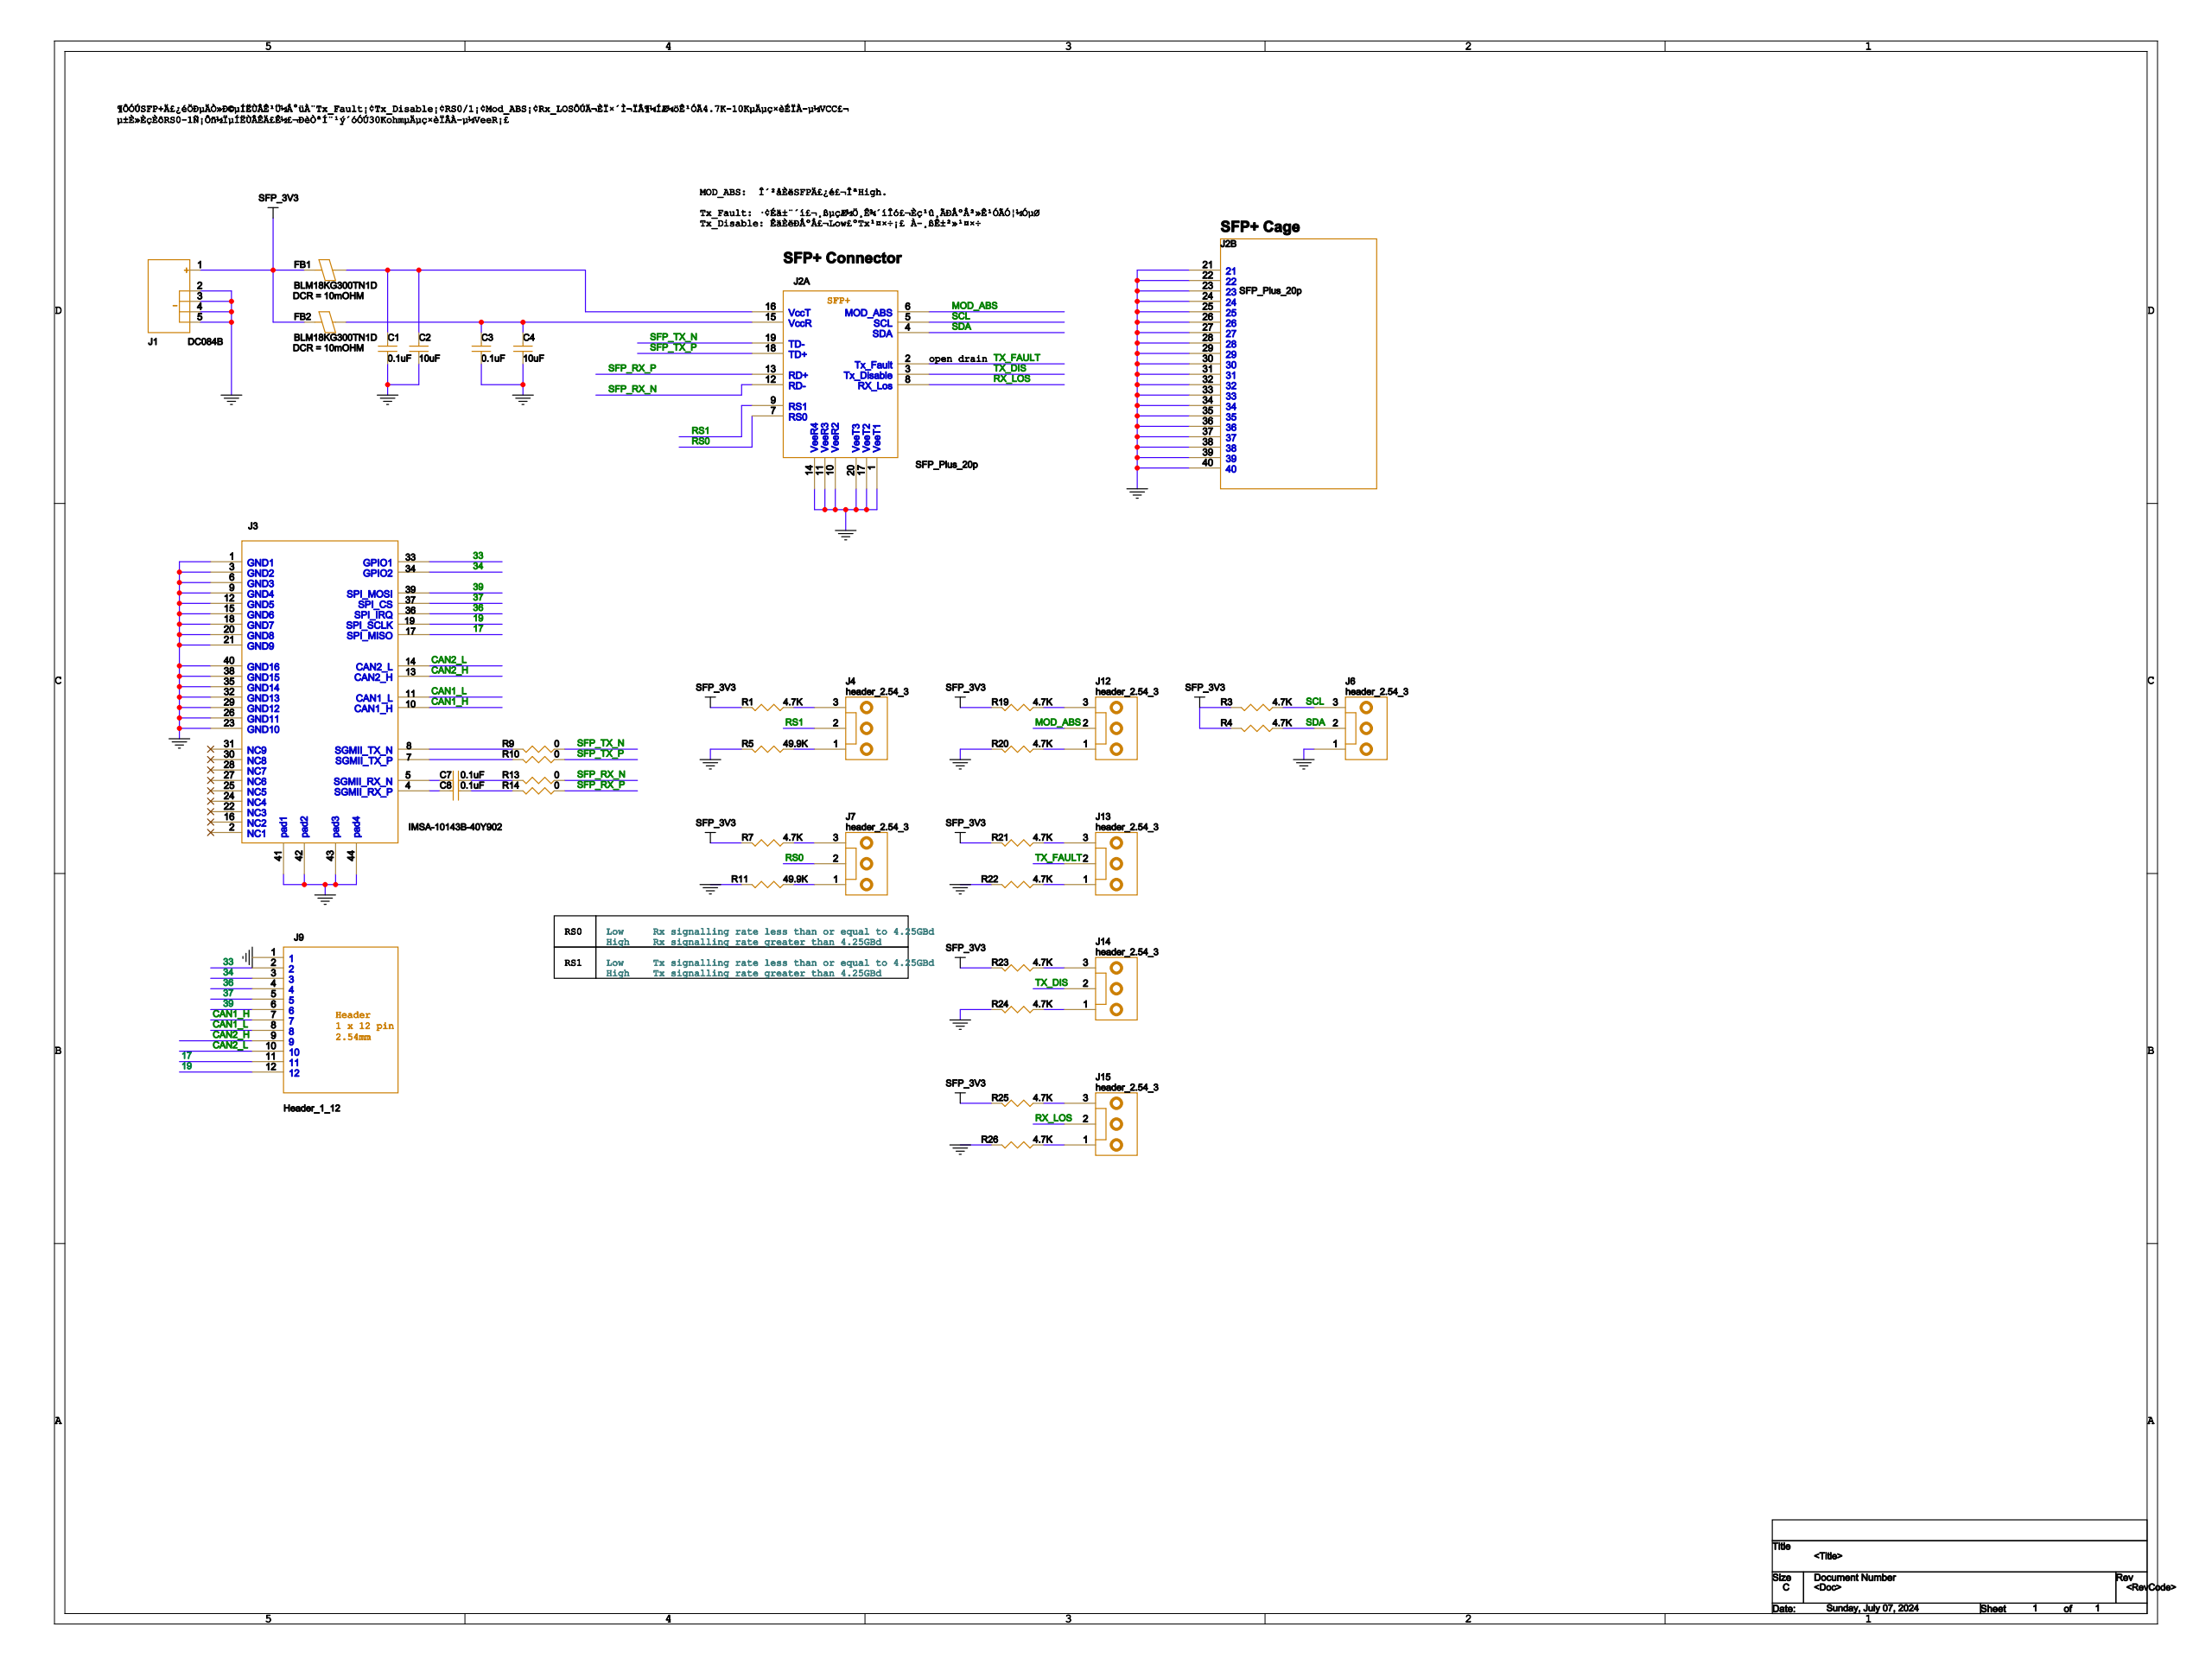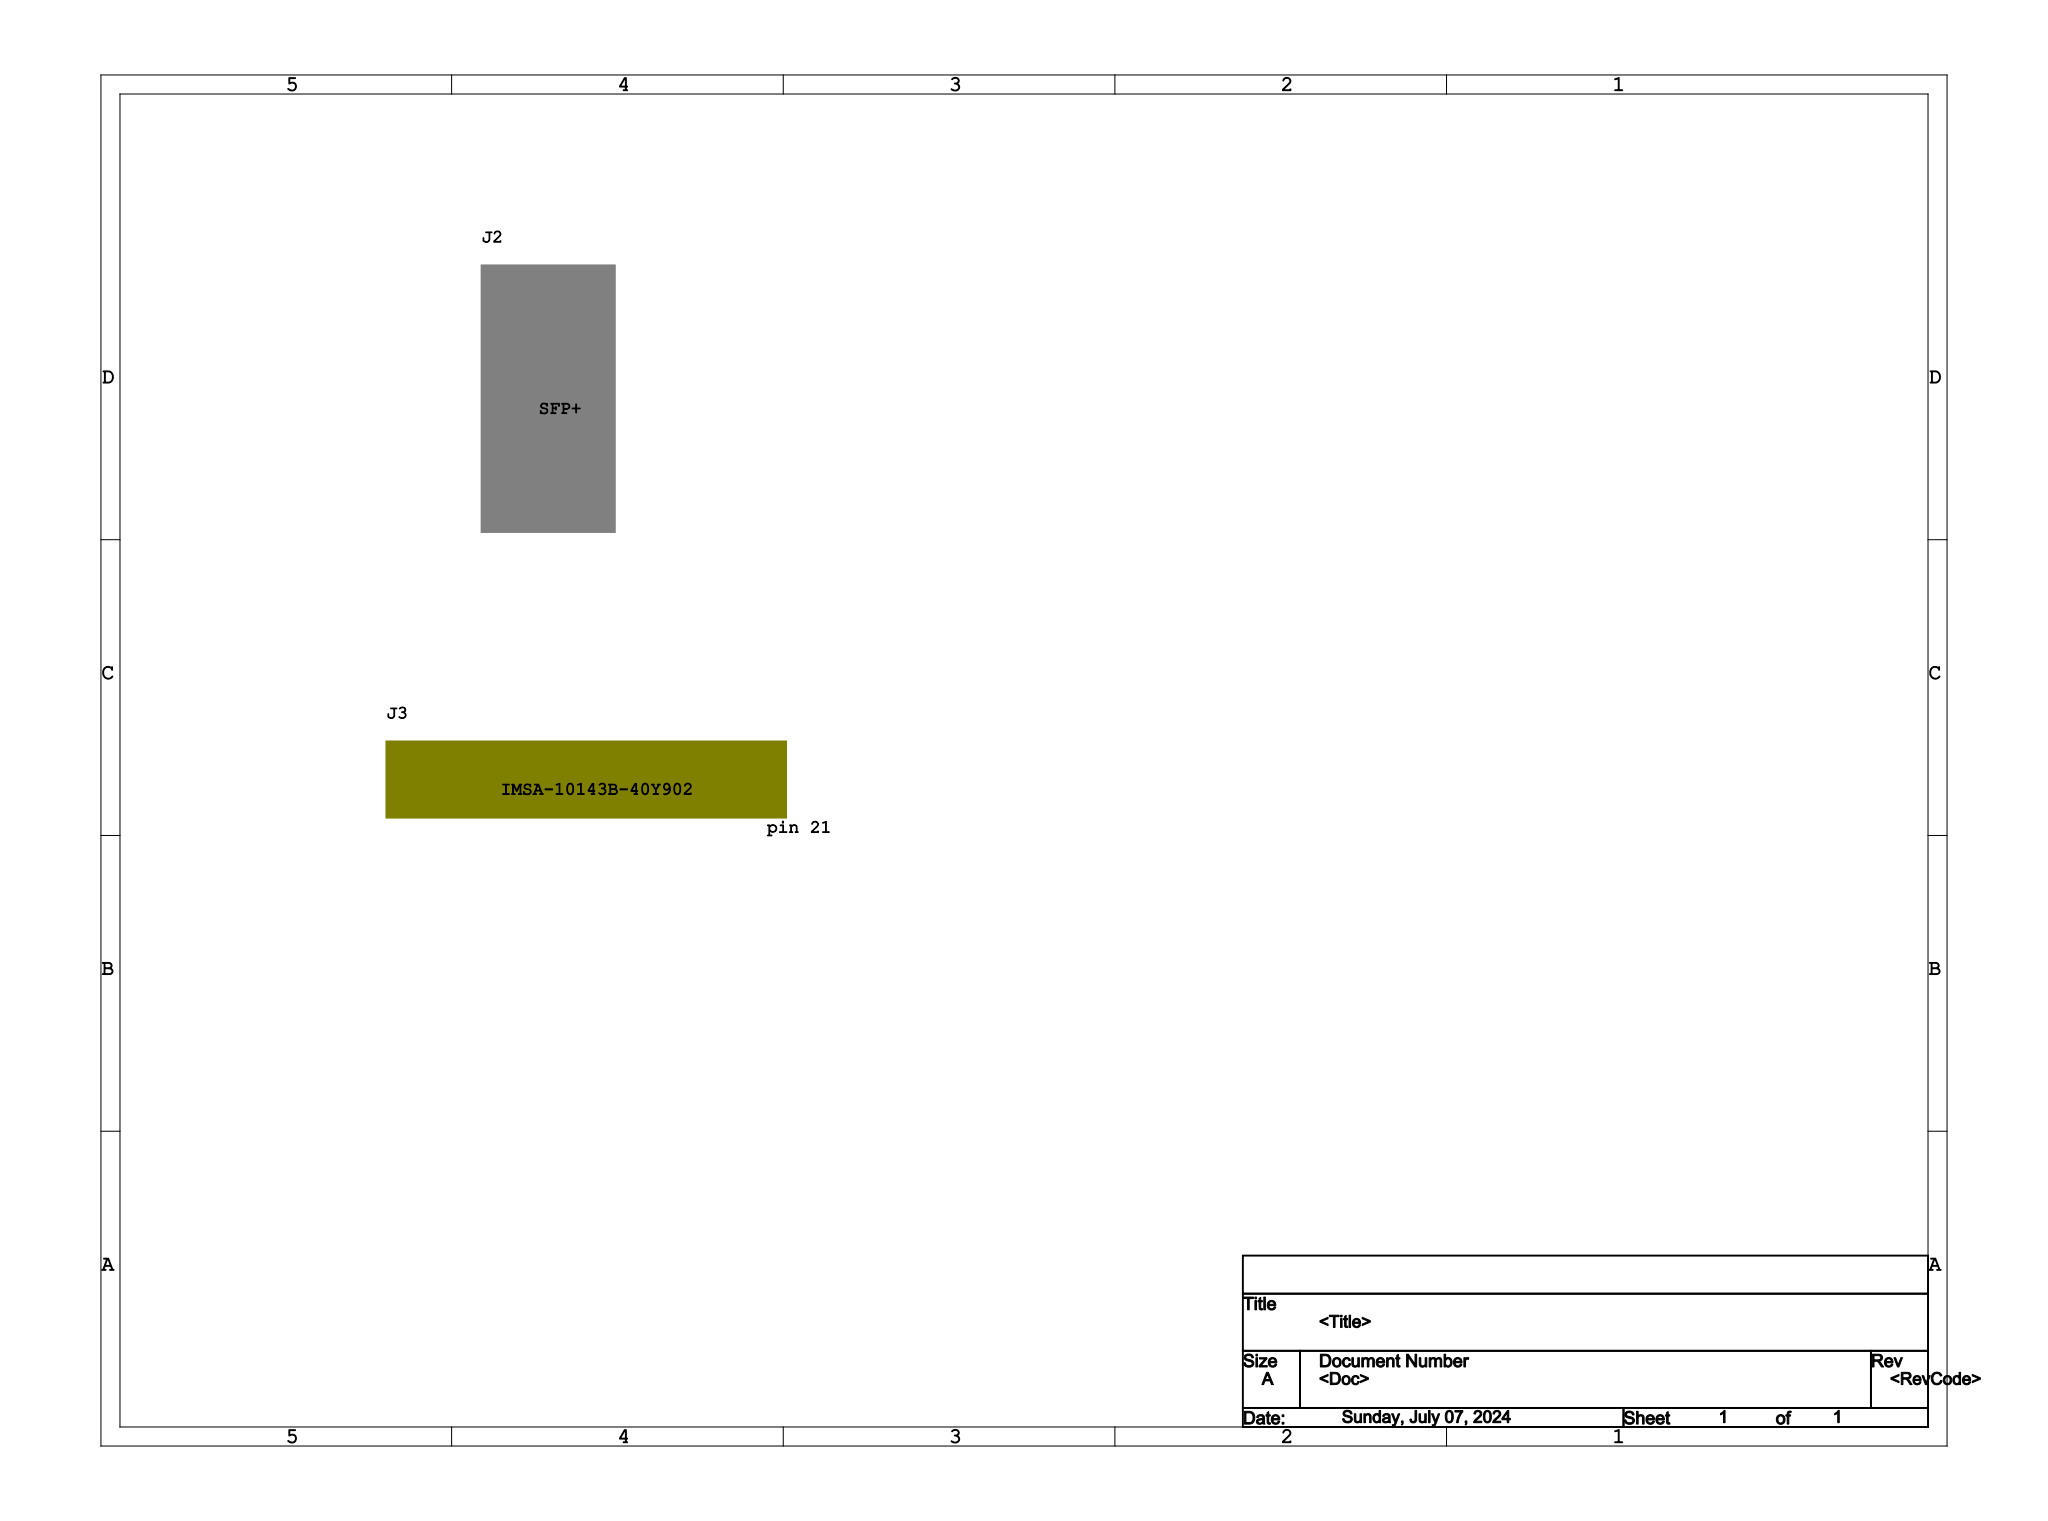Circuit board | Cadence Allegro | 37 parts | 45 nets
Bill of materials:
SYM_NAME,COMP_DEVICE_TYPE,COMP_VALUE,COMP_TOL,COMP_CLASS,REFDES
0603,CAP NP_0603_0.1UF,0.1uF,,DISCRETE,C1
0603,CAP NP_0603_10UF,10uF,,IC,C2
0603,CAP NP_0603_0.1UF,0.1uF,,DISCRETE,C3
0603,CAP NP_0603_10UF,10uF,,IC,C4
0603,CAP NP_0603_0.1UF,0.1uF,,DISCRETE,C7
0603,CAP NP_0603_0.1UF,0.1uF,,DISCRETE,C8
0603,002_FERRITE_0603_BLM18KG300TN1D,BLM18KG300TN1D,,IC,FB1
0603,002_FERRITE_0603_BLM18KG300TN1D,BLM18KG300TN1D,,IC,FB2
PWR5P_167X80_H78,DC084B_PWR5P_167X80_H78_DC084B,DC084B,,IC,J1
SFP_CAGE40P_490X161_H91,SFP_PLUS_20P_SFP_CAGE40P_490X16,SFP_Plus_20p,,IC,J2
BTB2X20P_205X74_05_H890_M,IMSA-10143B-40Y902_1_BTB2X20P_2,IMSA-10143B-40Y902,,IC,J3
003_HDR_KK,003_CONN_POL_003_HDR_KK_HEADER_,header_2.54_3,,IC,J4
003_HDR_KK,003_CONN_POL_003_HDR_KK_HEADER_,header_2.54_3,,IC,J6
003_HDR_KK,003_CONN_POL_003_HDR_KK_HEADER_,header_2.54_3,,IC,J7
DIP1X12,HEADER_1_12_DIP1X12_HEADER_1_12,Header_1_12,,IC,J9
003_HDR_KK,003_CONN_POL_003_HDR_KK_HEADER_,header_2.54_3,,IC,J12
003_HDR_KK,003_CONN_POL_003_HDR_KK_HEADER_,header_2.54_3,,IC,J13
003_HDR_KK,003_CONN_POL_003_HDR_KK_HEADER_,header_2.54_3,,IC,J14
003_HDR_KK,003_CONN_POL_003_HDR_KK_HEADER_,header_2.54_3,,IC,J15
0603,R_0_0603_4.7K,4.7K,,IC,R1
0603,R_0_0603_4.7K,4.7K,,IC,R3
0603,R_0_0603_4.7K,4.7K,,IC,R4
0603,R_0_0603_49.9K,49.9K,,IC,R5
0603,R_0_0603_4.7K,4.7K,,IC,R7
0603,R_0_0603_0,0,,DISCRETE,R9
0603,R_0_0603_0,0,,DISCRETE,R10
0603,R_0_0603_49.9K,49.9K,,IC,R11
0603,R_0_0603_0,0,,DISCRETE,R13
0603,R_0_0603_0,0,,DISCRETE,R14
0603,R_0_0603_4.7K,4.7K,,IC,R19
0603,R_0_0603_4.7K,4.7K,,IC,R20
0603,R_0_0603_4.7K,4.7K,,IC,R21
0603,R_0_0603_4.7K,4.7K,,IC,R22
0603,R_0_0603_4.7K,4.7K,,IC,R23
0603,R_0_0603_4.7K,4.7K,,IC,R24
0603,R_0_0603_4.7K,4.7K,,IC,R25
0603,R_0_0603_4.7K,4.7K,,IC,R26
Netlist (net: part-pin ...):
GND: C1-1 C2-1 C3-1 C4-1 J1-2 J1-3 J1-4 J1-5 J2-1 J2-10 J2-11 J2-14 J2-17 J2-20 J2-21 J2-22 J2-23 J2-24 J2-25 J2-26 J2-27 J2-28 J2-29 J2-30 J2-31 J2-32 J2-33 J2-34 J2-35 J2-36 J2-37 J2-38 J2-39 J2-40 J3-1 J3-3 J3-6 J3-9 J3-12 J3-15 J3-18 J3-20 J3-21 J3-23 J3-26 J3-29 J3-32 J3-35 J3-38 J3-40 J3-41 J3-42 J3-43 J3-44 J6-1 J9-1 R5-2 R11-2 R20-2 R22-2 R24-2 R26-2
CAN2_L: J3-14 J9-10
17: J3-17 J9-11
19: J3-19 J9-12
33: J3-33 J9-2
34: J3-34 J9-3
36: J3-36 J9-4
37: J3-37 J9-5
39: J3-39 J9-6
CAN1_H: J3-10 J9-7
CAN1_L: J3-11 J9-8
CAN2_H: J3-13 J9-9
N771454: C1-2 C2-2 FB1-1 J2-16
N771610: C3-2 C4-2 FB2-1 J2-15
N773415: C7-1 R13-2
N773411: C7-2 J3-5
N773473: C8-1 R14-2
N773433: C8-2 J3-4
SFP_3V3: FB1-2 FB2-2 J1-1 R1-2 R3-2 R4-2 R7-2 R19-2 R21-2 R23-2 R25-2
N812757: J12-1 R20-1
MOD_ABS: J2-6 J12-2
N812723: J12-3 R19-1
N812845: J13-1 R22-1
TX_FAULT: J2-2 J13-2
N812811: J13-3 R21-1
N813316: J14-1 R24-1
TX_DIS: J2-3 J14-2
N813282: J14-3 R23-1
N813404: J15-1 R26-1
RX_LOS: J2-8 J15-2
N813370: J15-3 R25-1
N779545: J4-1 R5-1
RS1: J2-9 J4-2
N779511: J4-3 R1-1
SDA: J2-4 J6-2 R4-1
SCL: J2-5 J6-3 R3-1
N797144: J7-1 R11-1
RS0: J2-7 J7-2
N779603: J7-3 R7-1
SFP_RX_P: J2-13 R14-1
SFP_RX_N: J2-12 R13-1
SFP_TX_P: J2-18 R10-1
SFP_TX_N: J2-19 R9-1
N773355: J3-8 R9-2
N773373: J3-7 R10-2